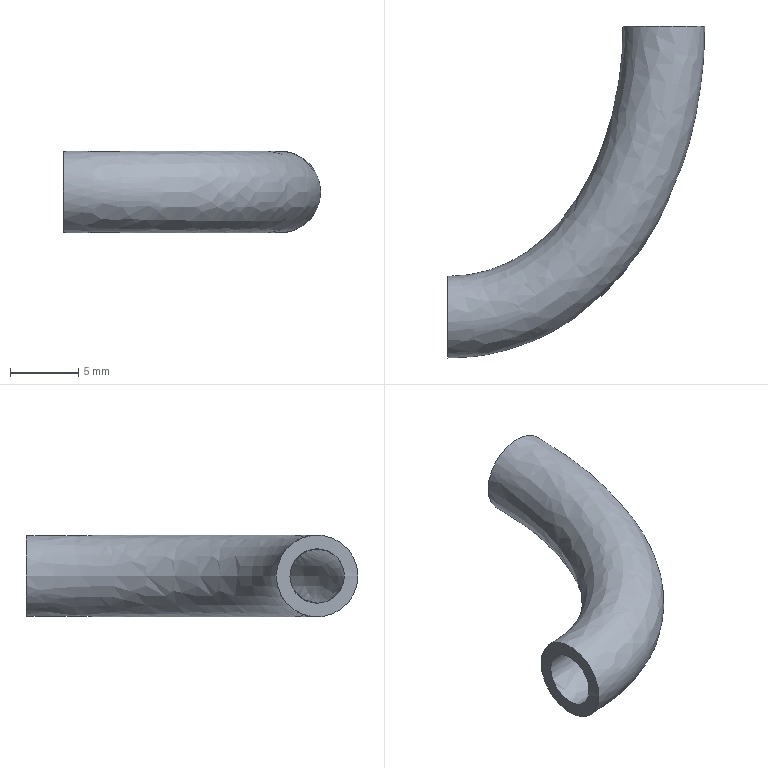Part | NX | features solid 2 | 1 solid | 4 faces | box 18.907 x 24.387 x 6 mm | volume 465.194 mm3 | plane 2 | spline 2